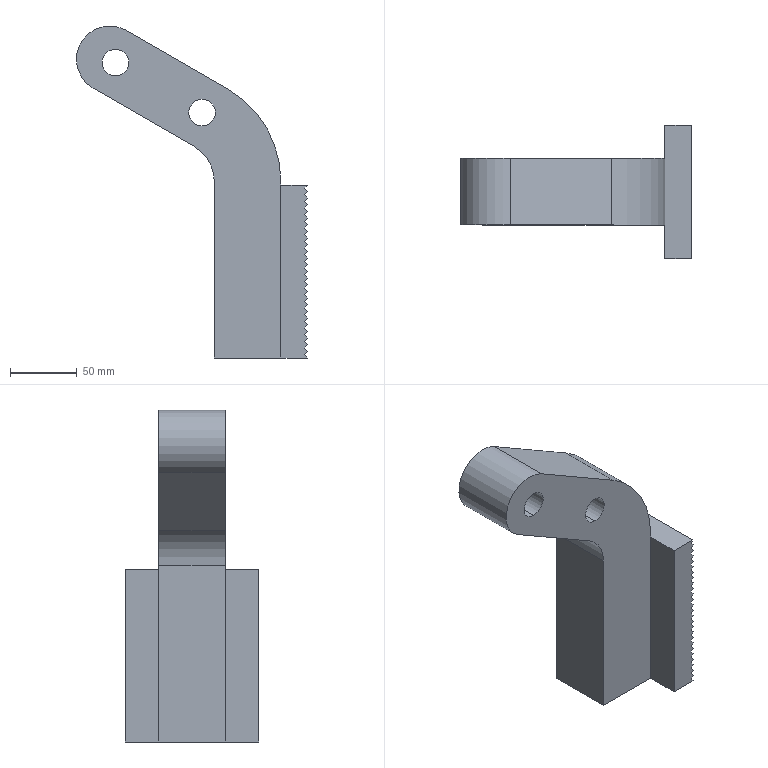Part | SolidWorks | features ICE 2, Extrusion 1, Fillet 1 | 1 solid | 71 faces | box 173.433 x 100 x 249.151 mm | volume 959009 mm3 | plane 64 | cylinder 7 | commonest cylinder face diameters 20 x4 50 x1 60 x1 160 x1